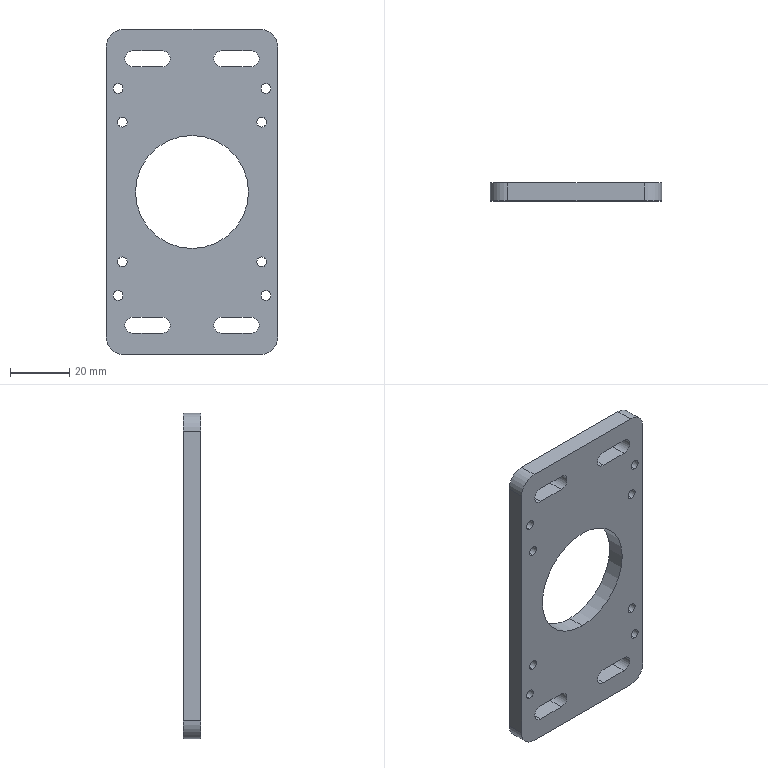Part | SolidWorks | features HoleWzd 2, Extrusion 1, ICE 1 | 1 solid | 44 faces | box 58 x 6 x 110 mm | volume 28962 mm3 | cylinder 30 | plane 14 | commonest cylinder face diameters 3.3 x16 5.4 x8 12 x4 38.2 x2
STEP:
#1=CARTESIAN_POINT('',(-25.,6.,36.65));
#2=VERTEX_POINT('',#1);
#3=CARTESIAN_POINT('',(-25.,6.,33.35));
#4=VERTEX_POINT('',#3);
#5=CARTESIAN_POINT('',(-25.,6.,35.));
#6=DIRECTION('',(0.,-1.,0.));
#7=DIRECTION('',(0.,0.,-1.));
#8=AXIS2_PLACEMENT_3D('',#5,#6,#7);
#9=CIRCLE('',#8,1.65);
#10=EDGE_CURVE('',#2,#4,#9,.T.);
#11=ORIENTED_EDGE('',*,*,#10,.F.);
#12=CARTESIAN_POINT('',(-25.,0.,36.65));
#13=VERTEX_POINT('',#12);
#14=CARTESIAN_POINT('',(-25.,0.,36.65));
#15=DIRECTION('',(0.,-1.,0.));
#16=VECTOR('',#15,1000.);
#17=LINE('',#14,#16);
#18=EDGE_CURVE('',#2,#13,#17,.T.);
#19=ORIENTED_EDGE('',*,*,#18,.T.);
#20=CARTESIAN_POINT('',(-25.,0.,33.35));
#21=VERTEX_POINT('',#20);
#22=CARTESIAN_POINT('',(-25.,0.,35.));
#23=DIRECTION('',(0.,-1.,0.));
#24=DIRECTION('',(0.,0.,-1.));
#25=AXIS2_PLACEMENT_3D('',#22,#23,#24);
#26=CIRCLE('',#25,1.65);
#27=EDGE_CURVE('',#13,#21,#26,.T.);
#28=ORIENTED_EDGE('',*,*,#27,.T.);
#29=CARTESIAN_POINT('',(-25.,0.,33.35));
#30=DIRECTION('',(0.,-1.,0.));
#31=VECTOR('',#30,1000.);
#32=LINE('',#29,#31);
#33=EDGE_CURVE('',#4,#21,#32,.T.);
#34=ORIENTED_EDGE('',*,*,#33,.F.);
#35=EDGE_LOOP('',(#11,#19,#28,#34));
#36=FACE_OUTER_BOUND('',#35,.T.);
#37=CARTESIAN_POINT('',(-25.,0.,35.));
#38=DIRECTION('',(0.,-1.,0.));
#39=DIRECTION('',(0.,0.,-1.));
#40=AXIS2_PLACEMENT_3D('',#37,#38,#39);
#41=CYLINDRICAL_SURFACE('',#40,1.65);
#42=ADVANCED_FACE('',(#36),#41,.F.);
#43=CARTESIAN_POINT('',(-25.,6.,-33.35));
#44=VERTEX_POINT('',#43);
#45=CARTESIAN_POINT('',(-25.,6.,-36.65));
#46=VERTEX_POINT('',#45);
#47=CARTESIAN_POINT('',(-25.,6.,-35.));
#48=DIRECTION('',(0.,-1.,0.));
#49=DIRECTION('',(0.,0.,-1.));
#50=AXIS2_PLACEMENT_3D('',#47,#48,#49);
#51=CIRCLE('',#50,1.65);
#52=EDGE_CURVE('',#44,#46,#51,.T.);
#53=ORIENTED_EDGE('',*,*,#52,.F.);
#54=CARTESIAN_POINT('',(-25.,0.,-33.35));
#55=VERTEX_POINT('',#54);
#56=CARTESIAN_POINT('',(-25.,0.,-33.35));
#57=DIRECTION('',(0.,-1.,0.));
#58=VECTOR('',#57,1000.);
#59=LINE('',#56,#58);
#60=EDGE_CURVE('',#44,#55,#59,.T.);
#61=ORIENTED_EDGE('',*,*,#60,.T.);
#62=CARTESIAN_POINT('',(-25.,0.,-36.65));
#63=VERTEX_POINT('',#62);
#64=CARTESIAN_POINT('',(-25.,0.,-35.));
#65=DIRECTION('',(0.,-1.,0.));
#66=DIRECTION('',(0.,0.,-1.));
#67=AXIS2_PLACEMENT_3D('',#64,#65,#66);
#68=CIRCLE('',#67,1.65);
#69=EDGE_CURVE('',#55,#63,#68,.T.);
#70=ORIENTED_EDGE('',*,*,#69,.T.);
#71=CARTESIAN_POINT('',(-25.,0.,-36.65));
#72=DIRECTION('',(0.,-1.,0.));
#73=VECTOR('',#72,1000.);
#74=LINE('',#71,#73);
#75=EDGE_CURVE('',#46,#63,#74,.T.);
#76=ORIENTED_EDGE('',*,*,#75,.F.);
#77=EDGE_LOOP('',(#53,#61,#70,#76));
#78=FACE_OUTER_BOUND('',#77,.T.);
#79=CARTESIAN_POINT('',(-25.,0.,-35.));
#80=DIRECTION('',(0.,-1.,0.));
#81=DIRECTION('',(0.,0.,-1.));
#82=AXIS2_PLACEMENT_3D('',#79,#80,#81);
#83=CYLINDRICAL_SURFACE('',#82,1.65);
#84=ADVANCED_FACE('',(#78),#83,.F.);
#85=CARTESIAN_POINT('',(25.,6.,-33.35));
#86=VERTEX_POINT('',#85);
#87=CARTESIAN_POINT('',(25.,6.,-36.65));
#88=VERTEX_POINT('',#87);
#89=CARTESIAN_POINT('',(25.,6.,-35.));
#90=DIRECTION('',(0.,-1.,0.));
#91=DIRECTION('',(0.,0.,-1.));
#92=AXIS2_PLACEMENT_3D('',#89,#90,#91);
#93=CIRCLE('',#92,1.65);
#94=EDGE_CURVE('',#86,#88,#93,.T.);
#95=ORIENTED_EDGE('',*,*,#94,.F.);
#96=CARTESIAN_POINT('',(25.,0.,-33.35));
#97=VERTEX_POINT('',#96);
#98=CARTESIAN_POINT('',(25.,0.,-33.35));
#99=DIRECTION('',(0.,-1.,0.));
#100=VECTOR('',#99,1000.);
#101=LINE('',#98,#100);
#102=EDGE_CURVE('',#86,#97,#101,.T.);
#103=ORIENTED_EDGE('',*,*,#102,.T.);
#104=CARTESIAN_POINT('',(25.,0.,-36.65));
#105=VERTEX_POINT('',#104);
#106=CARTESIAN_POINT('',(25.,0.,-35.));
#107=DIRECTION('',(0.,-1.,0.));
#108=DIRECTION('',(0.,0.,-1.));
#109=AXIS2_PLACEMENT_3D('',#106,#107,#108);
#110=CIRCLE('',#109,1.65);
#111=EDGE_CURVE('',#97,#105,#110,.T.);
#112=ORIENTED_EDGE('',*,*,#111,.T.);
#113=CARTESIAN_POINT('',(25.,0.,-36.65));
#114=DIRECTION('',(0.,-1.,0.));
#115=VECTOR('',#114,1000.);
#116=LINE('',#113,#115);
#117=EDGE_CURVE('',#88,#105,#116,.T.);
#118=ORIENTED_EDGE('',*,*,#117,.F.);
#119=EDGE_LOOP('',(#95,#103,#112,#118));
#120=FACE_OUTER_BOUND('',#119,.T.);
#121=CARTESIAN_POINT('',(25.,0.,-35.));
#122=DIRECTION('',(0.,-1.,0.));
#123=DIRECTION('',(0.,0.,-1.));
#124=AXIS2_PLACEMENT_3D('',#121,#122,#123);
#125=CYLINDRICAL_SURFACE('',#124,1.65);
#126=ADVANCED_FACE('',(#120),#125,.F.);
#127=CARTESIAN_POINT('',(25.,6.,36.65));
#128=VERTEX_POINT('',#127);
#129=CARTESIAN_POINT('',(25.,6.,33.35));
#130=VERTEX_POINT('',#129);
#131=CARTESIAN_POINT('',(25.,6.,35.));
#132=DIRECTION('',(0.,-1.,0.));
#133=DIRECTION('',(0.,0.,-1.));
#134=AXIS2_PLACEMENT_3D('',#131,#132,#133);
#135=CIRCLE('',#134,1.65);
#136=EDGE_CURVE('',#128,#130,#135,.T.);
#137=ORIENTED_EDGE('',*,*,#136,.F.);
#138=CARTESIAN_POINT('',(25.,0.,36.65));
#139=VERTEX_POINT('',#138);
#140=CARTESIAN_POINT('',(25.,0.,36.65));
#141=DIRECTION('',(0.,-1.,0.));
#142=VECTOR('',#141,1000.);
#143=LINE('',#140,#142);
#144=EDGE_CURVE('',#128,#139,#143,.T.);
#145=ORIENTED_EDGE('',*,*,#144,.T.);
#146=CARTESIAN_POINT('',(25.,0.,33.35));
#147=VERTEX_POINT('',#146);
#148=CARTESIAN_POINT('',(25.,0.,35.));
#149=DIRECTION('',(0.,-1.,0.));
#150=DIRECTION('',(0.,0.,-1.));
#151=AXIS2_PLACEMENT_3D('',#148,#149,#150);
#152=CIRCLE('',#151,1.65);
#153=EDGE_CURVE('',#139,#147,#152,.T.);
#154=ORIENTED_EDGE('',*,*,#153,.T.);
#155=CARTESIAN_POINT('',(25.,0.,33.35));
#156=DIRECTION('',(0.,-1.,0.));
#157=VECTOR('',#156,1000.);
#158=LINE('',#155,#157);
#159=EDGE_CURVE('',#130,#147,#158,.T.);
#160=ORIENTED_EDGE('',*,*,#159,.F.);
#161=EDGE_LOOP('',(#137,#145,#154,#160));
#162=FACE_OUTER_BOUND('',#161,.T.);
#163=CARTESIAN_POINT('',(25.,0.,35.));
#164=DIRECTION('',(0.,-1.,0.));
#165=DIRECTION('',(0.,0.,-1.));
#166=AXIS2_PLACEMENT_3D('',#163,#164,#165);
#167=CYLINDRICAL_SURFACE('',#166,1.65);
#168=ADVANCED_FACE('',(#162),#167,.F.);
#169=CARTESIAN_POINT('',(-23.57,0.,-21.92));
#170=VERTEX_POINT('',#169);
#171=CARTESIAN_POINT('',(-23.57,0.,-25.22));
#172=VERTEX_POINT('',#171);
#173=CARTESIAN_POINT('',(-23.57,0.,-23.57));
#174=DIRECTION('',(0.,-1.,0.));
#175=DIRECTION('',(0.,0.,-1.));
#176=AXIS2_PLACEMENT_3D('',#173,#174,#175);
#177=CIRCLE('',#176,1.65);
#178=EDGE_CURVE('',#170,#172,#177,.T.);
#179=ORIENTED_EDGE('',*,*,#178,.T.);
#180=CARTESIAN_POINT('',(-23.57,6.,-25.22));
#181=VERTEX_POINT('',#180);
#182=CARTESIAN_POINT('',(-23.57,6.,-25.22));
#183=DIRECTION('',(0.,1.,0.));
#184=VECTOR('',#183,1000.);
#185=LINE('',#182,#184);
#186=EDGE_CURVE('',#172,#181,#185,.T.);
#187=ORIENTED_EDGE('',*,*,#186,.T.);
#188=CARTESIAN_POINT('',(-23.57,6.,-21.92));
#189=VERTEX_POINT('',#188);
#190=CARTESIAN_POINT('',(-23.57,6.,-23.57));
#191=DIRECTION('',(0.,1.,0.));
#192=DIRECTION('',(0.,0.,1.));
#193=AXIS2_PLACEMENT_3D('',#190,#191,#192);
#194=CIRCLE('',#193,1.65);
#195=EDGE_CURVE('',#181,#189,#194,.T.);
#196=ORIENTED_EDGE('',*,*,#195,.T.);
#197=CARTESIAN_POINT('',(-23.57,6.,-21.92));
#198=DIRECTION('',(0.,1.,0.));
#199=VECTOR('',#198,1000.);
#200=LINE('',#197,#199);
#201=EDGE_CURVE('',#170,#189,#200,.T.);
#202=ORIENTED_EDGE('',*,*,#201,.F.);
#203=EDGE_LOOP('',(#179,#187,#196,#202));
#204=FACE_OUTER_BOUND('',#203,.T.);
#205=CARTESIAN_POINT('',(-23.57,6.,-23.57));
#206=DIRECTION('',(0.,1.,0.));
#207=DIRECTION('',(0.,0.,1.));
#208=AXIS2_PLACEMENT_3D('',#205,#206,#207);
#209=CYLINDRICAL_SURFACE('',#208,1.65);
#210=ADVANCED_FACE('',(#204),#209,.F.);
#211=CARTESIAN_POINT('',(23.57,0.,-21.92));
#212=VERTEX_POINT('',#211);
#213=CARTESIAN_POINT('',(23.57,0.,-25.22));
#214=VERTEX_POINT('',#213);
#215=CARTESIAN_POINT('',(23.57,0.,-23.57));
#216=DIRECTION('',(0.,-1.,0.));
#217=DIRECTION('',(0.,0.,-1.));
#218=AXIS2_PLACEMENT_3D('',#215,#216,#217);
#219=CIRCLE('',#218,1.65);
#220=EDGE_CURVE('',#212,#214,#219,.T.);
#221=ORIENTED_EDGE('',*,*,#220,.T.);
#222=CARTESIAN_POINT('',(23.57,6.,-25.22));
#223=VERTEX_POINT('',#222);
#224=CARTESIAN_POINT('',(23.57,6.,-25.22));
#225=DIRECTION('',(0.,1.,0.));
#226=VECTOR('',#225,1000.);
#227=LINE('',#224,#226);
#228=EDGE_CURVE('',#214,#223,#227,.T.);
#229=ORIENTED_EDGE('',*,*,#228,.T.);
#230=CARTESIAN_POINT('',(23.57,6.,-21.92));
#231=VERTEX_POINT('',#230);
#232=CARTESIAN_POINT('',(23.57,6.,-23.57));
#233=DIRECTION('',(0.,1.,0.));
#234=DIRECTION('',(0.,0.,1.));
#235=AXIS2_PLACEMENT_3D('',#232,#233,#234);
#236=CIRCLE('',#235,1.65);
#237=EDGE_CURVE('',#223,#231,#236,.T.);
#238=ORIENTED_EDGE('',*,*,#237,.T.);
#239=CARTESIAN_POINT('',(23.57,6.,-21.92));
#240=DIRECTION('',(0.,1.,0.));
#241=VECTOR('',#240,1000.);
#242=LINE('',#239,#241);
#243=EDGE_CURVE('',#212,#231,#242,.T.);
#244=ORIENTED_EDGE('',*,*,#243,.F.);
#245=EDGE_LOOP('',(#221,#229,#238,#244));
#246=FACE_OUTER_BOUND('',#245,.T.);
#247=CARTESIAN_POINT('',(23.57,6.,-23.57));
#248=DIRECTION('',(0.,1.,0.));
#249=DIRECTION('',(0.,0.,1.));
#250=AXIS2_PLACEMENT_3D('',#247,#248,#249);
#251=CYLINDRICAL_SURFACE('',#250,1.65);
#252=ADVANCED_FACE('',(#246),#251,.F.);
#253=CARTESIAN_POINT('',(23.57,0.,25.22));
#254=VERTEX_POINT('',#253);
#255=CARTESIAN_POINT('',(23.57,0.,21.92));
#256=VERTEX_POINT('',#255);
#257=CARTESIAN_POINT('',(23.57,0.,23.57));
#258=DIRECTION('',(0.,-1.,0.));
#259=DIRECTION('',(0.,0.,-1.));
#260=AXIS2_PLACEMENT_3D('',#257,#258,#259);
#261=CIRCLE('',#260,1.65);
#262=EDGE_CURVE('',#254,#256,#261,.T.);
#263=ORIENTED_EDGE('',*,*,#262,.T.);
#264=CARTESIAN_POINT('',(23.57,6.,21.92));
#265=VERTEX_POINT('',#264);
#266=CARTESIAN_POINT('',(23.57,6.,21.92));
#267=DIRECTION('',(0.,1.,0.));
#268=VECTOR('',#267,1000.);
#269=LINE('',#266,#268);
#270=EDGE_CURVE('',#256,#265,#269,.T.);
#271=ORIENTED_EDGE('',*,*,#270,.T.);
#272=CARTESIAN_POINT('',(23.57,6.,25.22));
#273=VERTEX_POINT('',#272);
#274=CARTESIAN_POINT('',(23.57,6.,23.57));
#275=DIRECTION('',(0.,1.,0.));
#276=DIRECTION('',(0.,0.,1.));
#277=AXIS2_PLACEMENT_3D('',#274,#275,#276);
#278=CIRCLE('',#277,1.65);
#279=EDGE_CURVE('',#265,#273,#278,.T.);
#280=ORIENTED_EDGE('',*,*,#279,.T.);
#281=CARTESIAN_POINT('',(23.57,6.,25.22));
#282=DIRECTION('',(0.,1.,0.));
#283=VECTOR('',#282,1000.);
#284=LINE('',#281,#283);
#285=EDGE_CURVE('',#254,#273,#284,.T.);
#286=ORIENTED_EDGE('',*,*,#285,.F.);
#287=EDGE_LOOP('',(#263,#271,#280,#286));
#288=FACE_OUTER_BOUND('',#287,.T.);
#289=CARTESIAN_POINT('',(23.57,6.,23.57));
#290=DIRECTION('',(0.,1.,0.));
#291=DIRECTION('',(0.,0.,1.));
#292=AXIS2_PLACEMENT_3D('',#289,#290,#291);
#293=CYLINDRICAL_SURFACE('',#292,1.65);
#294=ADVANCED_FACE('',(#288),#293,.F.);
#295=CARTESIAN_POINT('',(-23.57,0.,25.22));
#296=VERTEX_POINT('',#295);
#297=CARTESIAN_POINT('',(-23.57,0.,21.92));
#298=VERTEX_POINT('',#297);
#299=CARTESIAN_POINT('',(-23.57,0.,23.57));
#300=DIRECTION('',(0.,-1.,0.));
#301=DIRECTION('',(0.,0.,-1.));
#302=AXIS2_PLACEMENT_3D('',#299,#300,#301);
#303=CIRCLE('',#302,1.65);
#304=EDGE_CURVE('',#296,#298,#303,.T.);
#305=ORIENTED_EDGE('',*,*,#304,.T.);
#306=CARTESIAN_POINT('',(-23.57,6.,21.92));
#307=VERTEX_POINT('',#306);
#308=CARTESIAN_POINT('',(-23.57,6.,21.92));
#309=DIRECTION('',(0.,1.,0.));
#310=VECTOR('',#309,1000.);
#311=LINE('',#308,#310);
#312=EDGE_CURVE('',#298,#307,#311,.T.);
#313=ORIENTED_EDGE('',*,*,#312,.T.);
#314=CARTESIAN_POINT('',(-23.57,6.,25.22));
#315=VERTEX_POINT('',#314);
#316=CARTESIAN_POINT('',(-23.57,6.,23.57));
#317=DIRECTION('',(0.,1.,0.));
#318=DIRECTION('',(0.,0.,1.));
#319=AXIS2_PLACEMENT_3D('',#316,#317,#318);
#320=CIRCLE('',#319,1.65);
#321=EDGE_CURVE('',#307,#315,#320,.T.);
#322=ORIENTED_EDGE('',*,*,#321,.T.);
#323=CARTESIAN_POINT('',(-23.57,6.,25.22));
#324=DIRECTION('',(0.,1.,0.));
#325=VECTOR('',#324,1000.);
#326=LINE('',#323,#325);
#327=EDGE_CURVE('',#296,#315,#326,.T.);
#328=ORIENTED_EDGE('',*,*,#327,.F.);
#329=EDGE_LOOP('',(#305,#313,#322,#328));
#330=FACE_OUTER_BOUND('',#329,.T.);
#331=CARTESIAN_POINT('',(-23.57,6.,23.57));
#332=DIRECTION('',(0.,1.,0.));
#333=DIRECTION('',(0.,0.,1.));
#334=AXIS2_PLACEMENT_3D('',#331,#332,#333);
#335=CYLINDRICAL_SURFACE('',#334,1.65);
#336=ADVANCED_FACE('',(#330),#335,.F.);
#337=CARTESIAN_POINT('',(0.,6.,-19.1));
#338=VERTEX_POINT('',#337);
#339=CARTESIAN_POINT('',(0.,6.,19.1));
#340=VERTEX_POINT('',#339);
#341=CARTESIAN_POINT('',(0.,6.,0.));
#342=DIRECTION('',(0.,1.,0.));
#343=DIRECTION('',(0.,0.,1.));
#344=AXIS2_PLACEMENT_3D('',#341,#342,#343);
#345=CIRCLE('',#344,19.1);
#346=EDGE_CURVE('',#338,#340,#345,.T.);
#347=ORIENTED_EDGE('',*,*,#346,.T.);
#348=CARTESIAN_POINT('',(0.,0.,19.1));
#349=VERTEX_POINT('',#348);
#350=CARTESIAN_POINT('',(0.,6.,19.1));
#351=DIRECTION('',(0.,-1.,0.));
#352=VECTOR('',#351,1000.);
#353=LINE('',#350,#352);
#354=EDGE_CURVE('',#340,#349,#353,.T.);
#355=ORIENTED_EDGE('',*,*,#354,.T.);
#356=CARTESIAN_POINT('',(0.,0.,-19.1));
#357=VERTEX_POINT('',#356);
#358=CARTESIAN_POINT('',(0.,0.,0.));
#359=DIRECTION('',(0.,1.,0.));
#360=DIRECTION('',(0.,0.,1.));
#361=AXIS2_PLACEMENT_3D('',#358,#359,#360);
#362=CIRCLE('',#361,19.1);
#363=EDGE_CURVE('',#357,#349,#362,.T.);
#364=ORIENTED_EDGE('',*,*,#363,.F.);
#365=CARTESIAN_POINT('',(0.,6.,-19.1));
#366=DIRECTION('',(0.,-1.,0.));
#367=VECTOR('',#366,1000.);
#368=LINE('',#365,#367);
#369=EDGE_CURVE('',#338,#357,#368,.T.);
#370=ORIENTED_EDGE('',*,*,#369,.F.);
#371=EDGE_LOOP('',(#347,#355,#364,#370));
#372=FACE_OUTER_BOUND('',#371,.T.);
#373=CARTESIAN_POINT('',(0.,6.,0.));
#374=DIRECTION('',(0.,-1.,0.));
#375=DIRECTION('',(0.,0.,-1.));
#376=AXIS2_PLACEMENT_3D('',#373,#374,#375);
#377=CYLINDRICAL_SURFACE('',#376,19.1);
#378=ADVANCED_FACE('',(#372),#377,.F.);
#379=CARTESIAN_POINT('',(-25.,6.,35.));
#380=DIRECTION('',(0.,-1.,0.));
#381=DIRECTION('',(0.,0.,-1.));
#382=AXIS2_PLACEMENT_3D('',#379,#380,#381);
#383=CIRCLE('',#382,1.65);
#384=EDGE_CURVE('',#4,#2,#383,.T.);
#385=ORIENTED_EDGE('',*,*,#384,.T.);
#386=ORIENTED_EDGE('',*,*,#10,.T.);
#387=EDGE_LOOP('',(#385,#386));
#388=FACE_BOUND('',#387,.T.);
#389=CARTESIAN_POINT('',(-25.,6.,-35.));
#390=DIRECTION('',(0.,-1.,0.));
#391=DIRECTION('',(0.,0.,-1.));
#392=AXIS2_PLACEMENT_3D('',#389,#390,#391);
#393=CIRCLE('',#392,1.65);
#394=EDGE_CURVE('',#46,#44,#393,.T.);
#395=ORIENTED_EDGE('',*,*,#394,.T.);
#396=ORIENTED_EDGE('',*,*,#52,.T.);
#397=EDGE_LOOP('',(#395,#396));
#398=FACE_BOUND('',#397,.T.);
#399=CARTESIAN_POINT('',(25.,6.,-35.));
#400=DIRECTION('',(0.,-1.,0.));
#401=DIRECTION('',(0.,0.,-1.));
#402=AXIS2_PLACEMENT_3D('',#399,#400,#401);
#403=CIRCLE('',#402,1.65);
#404=EDGE_CURVE('',#88,#86,#403,.T.);
#405=ORIENTED_EDGE('',*,*,#404,.T.);
#406=ORIENTED_EDGE('',*,*,#94,.T.);
#407=EDGE_LOOP('',(#405,#406));
#408=FACE_BOUND('',#407,.T.);
#409=CARTESIAN_POINT('',(25.,6.,35.));
#410=DIRECTION('',(0.,-1.,0.));
#411=DIRECTION('',(0.,0.,-1.));
#412=AXIS2_PLACEMENT_3D('',#409,#410,#411);
#413=CIRCLE('',#412,1.65);
#414=EDGE_CURVE('',#130,#128,#413,.T.);
#415=ORIENTED_EDGE('',*,*,#414,.T.);
#416=ORIENTED_EDGE('',*,*,#136,.T.);
#417=EDGE_LOOP('',(#415,#416));
#418=FACE_BOUND('',#417,.T.);
#419=CARTESIAN_POINT('',(10.,6.,42.3));
#420=VERTEX_POINT('',#419);
#421=CARTESIAN_POINT('',(20.,6.,42.3));
#422=VERTEX_POINT('',#421);
#423=CARTESIAN_POINT('',(20.,6.,42.3));
#424=DIRECTION('',(1.,0.,0.));
#425=VECTOR('',#424,1000.);
#426=LINE('',#423,#425);
#427=EDGE_CURVE('',#420,#422,#426,.T.);
#428=ORIENTED_EDGE('',*,*,#427,.T.);
#429=CARTESIAN_POINT('',(20.,6.,47.7));
#430=VERTEX_POINT('',#429);
#431=CARTESIAN_POINT('',(20.,6.,45.));
#432=DIRECTION('',(0.,-1.,0.));
#433=DIRECTION('',(0.,0.,1.));
#434=AXIS2_PLACEMENT_3D('',#431,#432,#433);
#435=CIRCLE('',#434,2.7);
#436=EDGE_CURVE('',#422,#430,#435,.T.);
#437=ORIENTED_EDGE('',*,*,#436,.T.);
#438=CARTESIAN_POINT('',(10.,6.,47.7));
#439=VERTEX_POINT('',#438);
#440=CARTESIAN_POINT('',(20.,6.,47.7));
#441=DIRECTION('',(-1.,0.,0.));
#442=VECTOR('',#441,1000.);
#443=LINE('',#440,#442);
#444=EDGE_CURVE('',#430,#439,#443,.T.);
#445=ORIENTED_EDGE('',*,*,#444,.T.);
#446=CARTESIAN_POINT('',(10.,6.,45.));
#447=DIRECTION('',(0.,-1.,0.));
#448=DIRECTION('',(0.,0.,1.));
#449=AXIS2_PLACEMENT_3D('',#446,#447,#448);
#450=CIRCLE('',#449,2.7);
#451=EDGE_CURVE('',#439,#420,#450,.T.);
#452=ORIENTED_EDGE('',*,*,#451,.T.);
#453=EDGE_LOOP('',(#428,#437,#445,#452));
#454=FACE_BOUND('',#453,.T.);
#455=CARTESIAN_POINT('',(-10.,6.,-42.3));
#456=VERTEX_POINT('',#455);
#457=CARTESIAN_POINT('',(-20.,6.,-42.3));
#458=VERTEX_POINT('',#457);
#459=CARTESIAN_POINT('',(-20.,6.,-42.3));
#460=DIRECTION('',(-1.,0.,0.));
#461=VECTOR('',#460,1000.);
#462=LINE('',#459,#461);
#463=EDGE_CURVE('',#456,#458,#462,.T.);
#464=ORIENTED_EDGE('',*,*,#463,.T.);
#465=CARTESIAN_POINT('',(-20.,6.,-47.7));
#466=VERTEX_POINT('',#465);
#467=CARTESIAN_POINT('',(-20.,6.,-45.));
#468=DIRECTION('',(0.,-1.,0.));
#469=DIRECTION('',(0.,0.,1.));
#470=AXIS2_PLACEMENT_3D('',#467,#468,#469);
#471=CIRCLE('',#470,2.7);
#472=EDGE_CURVE('',#458,#466,#471,.T.);
#473=ORIENTED_EDGE('',*,*,#472,.T.);
#474=CARTESIAN_POINT('',(-10.,6.,-47.7));
#475=VERTEX_POINT('',#474);
#476=CARTESIAN_POINT('',(-20.,6.,-47.7));
#477=DIRECTION('',(1.,0.,0.));
#478=VECTOR('',#477,1000.);
#479=LINE('',#476,#478);
#480=EDGE_CURVE('',#466,#475,#479,.T.);
#481=ORIENTED_EDGE('',*,*,#480,.T.);
#482=CARTESIAN_POINT('',(-10.,6.,-45.));
#483=DIRECTION('',(0.,-1.,0.));
#484=DIRECTION('',(0.,0.,1.));
#485=AXIS2_PLACEMENT_3D('',#482,#483,#484);
#486=CIRCLE('',#485,2.7);
#487=EDGE_CURVE('',#475,#456,#486,.T.);
#488=ORIENTED_EDGE('',*,*,#487,.T.);
#489=EDGE_LOOP('',(#464,#473,#481,#488));
#490=FACE_BOUND('',#489,.T.);
#491=CARTESIAN_POINT('',(10.,6.,-47.7));
#492=VERTEX_POINT('',#491);
#493=CARTESIAN_POINT('',(20.,6.,-47.7));
#494=VERTEX_POINT('',#493);
#495=CARTESIAN_POINT('',(20.,6.,-47.7));
#496=DIRECTION('',(1.,0.,0.));
#497=VECTOR('',#496,1000.);
#498=LINE('',#495,#497);
#499=EDGE_CURVE('',#492,#494,#498,.T.);
#500=ORIENTED_EDGE('',*,*,#499,.T.);
#501=CARTESIAN_POINT('',(20.,6.,-42.3));
#502=VERTEX_POINT('',#501);
#503=CARTESIAN_POINT('',(20.,6.,-45.));
#504=DIRECTION('',(0.,-1.,0.));
#505=DIRECTION('',(0.,0.,-1.));
#506=AXIS2_PLACEMENT_3D('',#503,#504,#505);
#507=CIRCLE('',#506,2.7);
#508=EDGE_CURVE('',#494,#502,#507,.T.);
#509=ORIENTED_EDGE('',*,*,#508,.T.);
#510=CARTESIAN_POINT('',(10.,6.,-42.3));
#511=VERTEX_POINT('',#510);
#512=CARTESIAN_POINT('',(20.,6.,-42.3));
#513=DIRECTION('',(-1.,0.,0.));
#514=VECTOR('',#513,1000.);
#515=LINE('',#512,#514);
#516=EDGE_CURVE('',#502,#511,#515,.T.);
#517=ORIENTED_EDGE('',*,*,#516,.T.);
#518=CARTESIAN_POINT('',(10.,6.,-45.));
#519=DIRECTION('',(0.,-1.,0.));
#520=DIRECTION('',(0.,0.,-1.));
#521=AXIS2_PLACEMENT_3D('',#518,#519,#520);
#522=CIRCLE('',#521,2.7);
#523=EDGE_CURVE('',#511,#492,#522,.T.);
#524=ORIENTED_EDGE('',*,*,#523,.T.);
#525=EDGE_LOOP('',(#500,#509,#517,#524));
#526=FACE_BOUND('',#525,.T.);
#527=CARTESIAN_POINT('',(-10.,6.,47.7));
#528=VERTEX_POINT('',#527);
#529=CARTESIAN_POINT('',(-20.,6.,47.7));
#530=VERTEX_POINT('',#529);
#531=CARTESIAN_POINT('',(-20.,6.,47.7));
#532=DIRECTION('',(-1.,0.,0.));
#533=VECTOR('',#532,1000.);
#534=LINE('',#531,#533);
#535=EDGE_CURVE('',#528,#530,#534,.T.);
#536=ORIENTED_EDGE('',*,*,#535,.T.);
#537=CARTESIAN_POINT('',(-20.,6.,42.3));
#538=VERTEX_POINT('',#537);
#539=CARTESIAN_POINT('',(-20.,6.,45.));
#540=DIRECTION('',(0.,-1.,0.));
#541=DIRECTION('',(0.,0.,-1.));
#542=AXIS2_PLACEMENT_3D('',#539,#540,#541);
#543=CIRCLE('',#542,2.7);
#544=EDGE_CURVE('',#530,#538,#543,.T.);
#545=ORIENTED_EDGE('',*,*,#544,.T.);
#546=CARTESIAN_POINT('',(-10.,6.,42.3));
#547=VERTEX_POINT('',#546);
#548=CARTESIAN_POINT('',(-20.,6.,42.3));
#549=DIRECTION('',(1.,0.,0.));
#550=VECTOR('',#549,1000.);
#551=LINE('',#548,#550);
#552=EDGE_CURVE('',#538,#547,#551,.T.);
#553=ORIENTED_EDGE('',*,*,#552,.T.);
#554=CARTESIAN_POINT('',(-10.,6.,45.));
#555=DIRECTION('',(0.,-1.,0.));
#556=DIRECTION('',(0.,0.,-1.));
#557=AXIS2_PLACEMENT_3D('',#554,#555,#556);
#558=CIRCLE('',#557,2.7);
#559=EDGE_CURVE('',#547,#528,#558,.T.);
#560=ORIENTED_EDGE('',*,*,#559,.T.);
#561=EDGE_LOOP('',(#536,#545,#553,#560));
#562=FACE_BOUND('',#561,.T.);
#563=CARTESIAN_POINT('',(-23.57,6.,-23.57));
#564=DIRECTION('',(0.,1.,0.));
#565=DIRECTION('',(0.,0.,1.));
#566=AXIS2_PLACEMENT_3D('',#563,#564,#565);
#567=CIRCLE('',#566,1.65);
#568=EDGE_CURVE('',#189,#181,#567,.T.);
#569=ORIENTED_EDGE('',*,*,#568,.F.);
#570=ORIENTED_EDGE('',*,*,#195,.F.);
#571=EDGE_LOOP('',(#569,#570));
#572=FACE_BOUND('',#571,.T.);
#573=CARTESIAN_POINT('',(23.57,6.,-23.57));
#574=DIRECTION('',(0.,1.,0.));
#575=DIRECTION('',(0.,0.,1.));
#576=AXIS2_PLACEMENT_3D('',#573,#574,#575);
#577=CIRCLE('',#576,1.65);
#578=EDGE_CURVE('',#231,#223,#577,.T.);
#579=ORIENTED_EDGE('',*,*,#578,.F.);
#580=ORIENTED_EDGE('',*,*,#237,.F.);
#581=EDGE_LOOP('',(#579,#580));
#582=FACE_BOUND('',#581,.T.);
#583=CARTESIAN_POINT('',(23.57,6.,23.57));
#584=DIRECTION('',(0.,1.,0.));
#585=DIRECTION('',(0.,0.,1.));
#586=AXIS2_PLACEMENT_3D('',#583,#584,#585);
#587=CIRCLE('',#586,1.65);
#588=EDGE_CURVE('',#273,#265,#587,.T.);
#589=ORIENTED_EDGE('',*,*,#588,.F.);
#590=ORIENTED_EDGE('',*,*,#279,.F.);
#591=EDGE_LOOP('',(#589,#590));
#592=FACE_BOUND('',#591,.T.);
#593=CARTESIAN_POINT('',(-23.57,6.,23.57));
#594=DIRECTION('',(0.,1.,0.));
#595=DIRECTION('',(0.,0.,1.));
#596=AXIS2_PLACEMENT_3D('',#593,#594,#595);
#597=CIRCLE('',#596,1.65);
#598=EDGE_CURVE('',#315,#307,#597,.T.);
#599=ORIENTED_EDGE('',*,*,#598,.F.);
#600=ORIENTED_EDGE('',*,*,#321,.F.);
#601=EDGE_LOOP('',(#599,#600));
#602=FACE_BOUND('',#601,.T.);
#603=CARTESIAN_POINT('',(29.,6.,-49.));
#604=VERTEX_POINT('',#603);
#605=CARTESIAN_POINT('',(23.,6.,-55.));
#606=VERTEX_POINT('',#605);
#607=CARTESIAN_POINT('',(23.,6.,-49.));
#608=DIRECTION('',(0.,1.,0.));
#609=DIRECTION('',(0.,0.,-1.));
#610=AXIS2_PLACEMENT_3D('',#607,#608,#609);
#611=CIRCLE('',#610,6.);
#612=EDGE_CURVE('',#604,#606,#611,.T.);
#613=ORIENTED_EDGE('',*,*,#612,.T.);
#614=CARTESIAN_POINT('',(-23.,6.,-55.));
#615=VERTEX_POINT('',#614);
#616=CARTESIAN_POINT('',(-23.,6.,-55.));
#617=DIRECTION('',(-1.,0.,0.));
#618=VECTOR('',#617,1000.);
#619=LINE('',#616,#618);
#620=EDGE_CURVE('',#606,#615,#619,.T.);
#621=ORIENTED_EDGE('',*,*,#620,.T.);
#622=CARTESIAN_POINT('',(-29.,6.,-49.));
#623=VERTEX_POINT('',#622);
#624=CARTESIAN_POINT('',(-23.,6.,-49.));
#625=DIRECTION('',(0.,1.,0.));
#626=DIRECTION('',(0.,0.,1.));
#627=AXIS2_PLACEMENT_3D('',#624,#625,#626);
#628=CIRCLE('',#627,6.);
#629=EDGE_CURVE('',#615,#623,#628,.T.);
#630=ORIENTED_EDGE('',*,*,#629,.T.);
#631=CARTESIAN_POINT('',(-29.,6.,49.));
#632=VERTEX_POINT('',#631);
#633=CARTESIAN_POINT('',(-29.,6.,-49.));
#634=DIRECTION('',(0.,0.,1.));
#635=VECTOR('',#634,1000.);
#636=LINE('',#633,#635);
#637=EDGE_CURVE('',#623,#632,#636,.T.);
#638=ORIENTED_EDGE('',*,*,#637,.T.);
#639=CARTESIAN_POINT('',(-23.,6.,55.));
#640=VERTEX_POINT('',#639);
#641=CARTESIAN_POINT('',(-23.,6.,49.));
#642=DIRECTION('',(0.,1.,0.));
#643=DIRECTION('',(0.,0.,1.));
#644=AXIS2_PLACEMENT_3D('',#641,#642,#643);
#645=CIRCLE('',#644,6.);
#646=EDGE_CURVE('',#632,#640,#645,.T.);
#647=ORIENTED_EDGE('',*,*,#646,.T.);
#648=CARTESIAN_POINT('',(23.,6.,55.));
#649=VERTEX_POINT('',#648);
#650=CARTESIAN_POINT('',(-23.,6.,55.));
#651=DIRECTION('',(1.,0.,0.));
#652=VECTOR('',#651,1000.);
#653=LINE('',#650,#652);
#654=EDGE_CURVE('',#640,#649,#653,.T.);
#655=ORIENTED_EDGE('',*,*,#654,.T.);
#656=CARTESIAN_POINT('',(29.,6.,49.));
#657=VERTEX_POINT('',#656);
#658=CARTESIAN_POINT('',(23.,6.,49.));
#659=DIRECTION('',(0.,1.,0.));
#660=DIRECTION('',(0.,0.,1.));
#661=AXIS2_PLACEMENT_3D('',#658,#659,#660);
#662=CIRCLE('',#661,6.);
#663=EDGE_CURVE('',#649,#657,#662,.T.);
#664=ORIENTED_EDGE('',*,*,#663,.T.);
#665=CARTESIAN_POINT('',(29.,6.,-49.));
#666=DIRECTION('',(0.,0.,-1.));
#667=VECTOR('',#666,1000.);
#668=LINE('',#665,#667);
#669=EDGE_CURVE('',#657,#604,#668,.T.);
#670=ORIENTED_EDGE('',*,*,#669,.T.);
#671=EDGE_LOOP('',(#613,#621,#630,#638,#647,#655,#664,#670));
#672=FACE_OUTER_BOUND('',#671,.T.);
#673=ORIENTED_EDGE('',*,*,#346,.F.);
#674=CARTESIAN_POINT('',(0.,6.,0.));
#675=DIRECTION('',(0.,1.,0.));
#676=DIRECTION('',(0.,0.,1.));
#677=AXIS2_PLACEMENT_3D('',#674,#675,#676);
#678=CIRCLE('',#677,19.1);
#679=EDGE_CURVE('',#340,#338,#678,.T.);
#680=ORIENTED_EDGE('',*,*,#679,.F.);
#681=EDGE_LOOP('',(#673,#680));
#682=FACE_BOUND('',#681,.T.);
#683=CARTESIAN_POINT('',(23.,6.,-49.));
#684=DIRECTION('',(0.,-1.,0.));
#685=DIRECTION('',(0.,0.,-1.));
#686=AXIS2_PLACEMENT_3D('',#683,#684,#685);
#687=PLANE('',#686);
#688=ADVANCED_FACE('',(#388,#398,#408,#418,#454,#490,#526,#562,#572,#582,#592,#602,#672,#682),#687,.F.);
#689=CARTESIAN_POINT('',(-25.,0.,35.));
#690=DIRECTION('',(0.,-1.,0.));
#691=DIRECTION('',(0.,0.,-1.));
#692=AXIS2_PLACEMENT_3D('',#689,#690,#691);
#693=CIRCLE('',#692,1.65);
#694=EDGE_CURVE('',#21,#13,#693,.T.);
#695=ORIENTED_EDGE('',*,*,#694,.F.);
#696=ORIENTED_EDGE('',*,*,#27,.F.);
#697=EDGE_LOOP('',(#695,#696));
#698=FACE_BOUND('',#697,.T.);
#699=CARTESIAN_POINT('',(-25.,0.,-35.));
#700=DIRECTION('',(0.,-1.,0.));
#701=DIRECTION('',(0.,0.,-1.));
#702=AXIS2_PLACEMENT_3D('',#699,#700,#701);
#703=CIRCLE('',#702,1.65);
#704=EDGE_CURVE('',#63,#55,#703,.T.);
#705=ORIENTED_EDGE('',*,*,#704,.F.);
#706=ORIENTED_EDGE('',*,*,#69,.F.);
#707=EDGE_LOOP('',(#705,#706));
#708=FACE_BOUND('',#707,.T.);
#709=CARTESIAN_POINT('',(25.,0.,-35.));
#710=DIRECTION('',(0.,-1.,0.));
#711=DIRECTION('',(0.,0.,-1.));
#712=AXIS2_PLACEMENT_3D('',#709,#710,#711);
#713=CIRCLE('',#712,1.65);
#714=EDGE_CURVE('',#105,#97,#713,.T.);
#715=ORIENTED_EDGE('',*,*,#714,.F.);
#716=ORIENTED_EDGE('',*,*,#111,.F.);
#717=EDGE_LOOP('',(#715,#716));
#718=FACE_BOUND('',#717,.T.);
#719=CARTESIAN_POINT('',(25.,0.,35.));
#720=DIRECTION('',(0.,-1.,0.));
#721=DIRECTION('',(0.,0.,-1.));
#722=AXIS2_PLACEMENT_3D('',#719,#720,#721);
#723=CIRCLE('',#722,1.65);
#724=EDGE_CURVE('',#147,#139,#723,.T.);
#725=ORIENTED_EDGE('',*,*,#724,.F.);
#726=ORIENTED_EDGE('',*,*,#153,.F.);
#727=EDGE_LOOP('',(#725,#726));
#728=FACE_BOUND('',#727,.T.);
#729=CARTESIAN_POINT('',(20.,0.,42.3));
#730=VERTEX_POINT('',#729);
#731=CARTESIAN_POINT('',(20.,0.,47.7));
#732=VERTEX_POINT('',#731);
#733=CARTESIAN_POINT('',(20.,0.,45.));
#734=DIRECTION('',(0.,-1.,0.));
#735=DIRECTION('',(0.,0.,1.));
#736=AXIS2_PLACEMENT_3D('',#733,#734,#735);
#737=CIRCLE('',#736,2.7);
#738=EDGE_CURVE('',#730,#732,#737,.T.);
#739=ORIENTED_EDGE('',*,*,#738,.F.);
#740=CARTESIAN_POINT('',(10.,0.,42.3));
#741=VERTEX_POINT('',#740);
#742=CARTESIAN_POINT('',(20.,0.,42.3));
#743=DIRECTION('',(1.,0.,0.));
#744=VECTOR('',#743,1000.);
#745=LINE('',#742,#744);
#746=EDGE_CURVE('',#741,#730,#745,.T.);
#747=ORIENTED_EDGE('',*,*,#746,.F.);
#748=CARTESIAN_POINT('',(10.,0.,47.7));
#749=VERTEX_POINT('',#748);
#750=CARTESIAN_POINT('',(10.,0.,45.));
#751=DIRECTION('',(0.,-1.,0.));
#752=DIRECTION('',(0.,0.,1.));
#753=AXIS2_PLACEMENT_3D('',#750,#751,#752);
#754=CIRCLE('',#753,2.7);
#755=EDGE_CURVE('',#749,#741,#754,.T.);
#756=ORIENTED_EDGE('',*,*,#755,.F.);
#757=CARTESIAN_POINT('',(20.,0.,47.7));
#758=DIRECTION('',(-1.,0.,0.));
#759=VECTOR('',#758,1000.);
#760=LINE('',#757,#759);
#761=EDGE_CURVE('',#732,#749,#760,.T.);
#762=ORIENTED_EDGE('',*,*,#761,.F.);
#763=EDGE_LOOP('',(#739,#747,#756,#762));
#764=FACE_BOUND('',#763,.T.);
#765=CARTESIAN_POINT('',(-20.,0.,-42.3));
#766=VERTEX_POINT('',#765);
#767=CARTESIAN_POINT('',(-20.,0.,-47.7));
#768=VERTEX_POINT('',#767);
#769=CARTESIAN_POINT('',(-20.,0.,-45.));
#770=DIRECTION('',(0.,-1.,0.));
#771=DIRECTION('',(0.,0.,1.));
#772=AXIS2_PLACEMENT_3D('',#769,#770,#771);
#773=CIRCLE('',#772,2.7);
#774=EDGE_CURVE('',#766,#768,#773,.T.);
#775=ORIENTED_EDGE('',*,*,#774,.F.);
#776=CARTESIAN_POINT('',(-10.,0.,-42.3));
#777=VERTEX_POINT('',#776);
#778=CARTESIAN_POINT('',(-20.,0.,-42.3));
#779=DIRECTION('',(-1.,0.,0.));
#780=VECTOR('',#779,1000.);
#781=LINE('',#778,#780);
#782=EDGE_CURVE('',#777,#766,#781,.T.);
#783=ORIENTED_EDGE('',*,*,#782,.F.);
#784=CARTESIAN_POINT('',(-10.,0.,-47.7));
#785=VERTEX_POINT('',#784);
#786=CARTESIAN_POINT('',(-10.,0.,-45.));
#787=DIRECTION('',(0.,-1.,0.));
#788=DIRECTION('',(0.,0.,1.));
#789=AXIS2_PLACEMENT_3D('',#786,#787,#788);
#790=CIRCLE('',#789,2.7);
#791=EDGE_CURVE('',#785,#777,#790,.T.);
#792=ORIENTED_EDGE('',*,*,#791,.F.);
#793=CARTESIAN_POINT('',(-20.,0.,-47.7));
#794=DIRECTION('',(1.,0.,0.));
#795=VECTOR('',#794,1000.);
#796=LINE('',#793,#795);
#797=EDGE_CURVE('',#768,#785,#796,.T.);
#798=ORIENTED_EDGE('',*,*,#797,.F.);
#799=EDGE_LOOP('',(#775,#783,#792,#798));
#800=FACE_BOUND('',#799,.T.);
#801=CARTESIAN_POINT('',(20.,0.,-47.7));
#802=VERTEX_POINT('',#801);
#803=CARTESIAN_POINT('',(20.,0.,-42.3));
#804=VERTEX_POINT('',#803);
#805=CARTESIAN_POINT('',(20.,0.,-45.));
#806=DIRECTION('',(0.,-1.,0.));
#807=DIRECTION('',(0.,0.,-1.));
#808=AXIS2_PLACEMENT_3D('',#805,#806,#807);
#809=CIRCLE('',#808,2.7);
#810=EDGE_CURVE('',#802,#804,#809,.T.);
#811=ORIENTED_EDGE('',*,*,#810,.F.);
#812=CARTESIAN_POINT('',(10.,0.,-47.7));
#813=VERTEX_POINT('',#812);
#814=CARTESIAN_POINT('',(20.,0.,-47.7));
#815=DIRECTION('',(1.,0.,0.));
#816=VECTOR('',#815,1000.);
#817=LINE('',#814,#816);
#818=EDGE_CURVE('',#813,#802,#817,.T.);
#819=ORIENTED_EDGE('',*,*,#818,.F.);
#820=CARTESIAN_POINT('',(10.,0.,-42.3));
#821=VERTEX_POINT('',#820);
#822=CARTESIAN_POINT('',(10.,0.,-45.));
#823=DIRECTION('',(0.,-1.,0.));
#824=DIRECTION('',(0.,0.,-1.));
#825=AXIS2_PLACEMENT_3D('',#822,#823,#824);
#826=CIRCLE('',#825,2.7);
#827=EDGE_CURVE('',#821,#813,#826,.T.);
#828=ORIENTED_EDGE('',*,*,#827,.F.);
#829=CARTESIAN_POINT('',(20.,0.,-42.3));
#830=DIRECTION('',(-1.,0.,0.));
#831=VECTOR('',#830,1000.);
#832=LINE('',#829,#831);
#833=EDGE_CURVE('',#804,#821,#832,.T.);
#834=ORIENTED_EDGE('',*,*,#833,.F.);
#835=EDGE_LOOP('',(#811,#819,#828,#834));
#836=FACE_BOUND('',#835,.T.);
#837=CARTESIAN_POINT('',(-20.,0.,47.7));
#838=VERTEX_POINT('',#837);
#839=CARTESIAN_POINT('',(-20.,0.,42.3));
#840=VERTEX_POINT('',#839);
#841=CARTESIAN_POINT('',(-20.,0.,45.));
#842=DIRECTION('',(0.,-1.,0.));
#843=DIRECTION('',(0.,0.,-1.));
#844=AXIS2_PLACEMENT_3D('',#841,#842,#843);
#845=CIRCLE('',#844,2.7);
#846=EDGE_CURVE('',#838,#840,#845,.T.);
#847=ORIENTED_EDGE('',*,*,#846,.F.);
#848=CARTESIAN_POINT('',(-10.,0.,47.7));
#849=VERTEX_POINT('',#848);
#850=CARTESIAN_POINT('',(-20.,0.,47.7));
#851=DIRECTION('',(-1.,0.,0.));
#852=VECTOR('',#851,1000.);
#853=LINE('',#850,#852);
#854=EDGE_CURVE('',#849,#838,#853,.T.);
#855=ORIENTED_EDGE('',*,*,#854,.F.);
#856=CARTESIAN_POINT('',(-10.,0.,42.3));
#857=VERTEX_POINT('',#856);
#858=CARTESIAN_POINT('',(-10.,0.,45.));
#859=DIRECTION('',(0.,-1.,0.));
#860=DIRECTION('',(0.,0.,-1.));
#861=AXIS2_PLACEMENT_3D('',#858,#859,#860);
#862=CIRCLE('',#861,2.7);
#863=EDGE_CURVE('',#857,#849,#862,.T.);
#864=ORIENTED_EDGE('',*,*,#863,.F.);
#865=CARTESIAN_POINT('',(-20.,0.,42.3));
#866=DIRECTION('',(1.,0.,0.));
#867=VECTOR('',#866,1000.);
#868=LINE('',#865,#867);
#869=EDGE_CURVE('',#840,#857,#868,.T.);
#870=ORIENTED_EDGE('',*,*,#869,.F.);
#871=EDGE_LOOP('',(#847,#855,#864,#870));
#872=FACE_BOUND('',#871,.T.);
#873=ORIENTED_EDGE('',*,*,#178,.F.);
#874=CARTESIAN_POINT('',(-23.57,0.,-23.57));
#875=DIRECTION('',(0.,-1.,0.));
#876=DIRECTION('',(0.,0.,-1.));
#877=AXIS2_PLACEMENT_3D('',#874,#875,#876);
#878=CIRCLE('',#877,1.65);
#879=EDGE_CURVE('',#172,#170,#878,.T.);
#880=ORIENTED_EDGE('',*,*,#879,.F.);
#881=EDGE_LOOP('',(#873,#880));
#882=FACE_BOUND('',#881,.T.);
#883=ORIENTED_EDGE('',*,*,#220,.F.);
#884=CARTESIAN_POINT('',(23.57,0.,-23.57));
#885=DIRECTION('',(0.,-1.,0.));
#886=DIRECTION('',(0.,0.,-1.));
#887=AXIS2_PLACEMENT_3D('',#884,#885,#886);
#888=CIRCLE('',#887,1.65);
#889=EDGE_CURVE('',#214,#212,#888,.T.);
#890=ORIENTED_EDGE('',*,*,#889,.F.);
#891=EDGE_LOOP('',(#883,#890));
#892=FACE_BOUND('',#891,.T.);
#893=ORIENTED_EDGE('',*,*,#262,.F.);
#894=CARTESIAN_POINT('',(23.57,0.,23.57));
#895=DIRECTION('',(0.,-1.,0.));
#896=DIRECTION('',(0.,0.,-1.));
#897=AXIS2_PLACEMENT_3D('',#894,#895,#896);
#898=CIRCLE('',#897,1.65);
#899=EDGE_CURVE('',#256,#254,#898,.T.);
#900=ORIENTED_EDGE('',*,*,#899,.F.);
#901=EDGE_LOOP('',(#893,#900));
#902=FACE_BOUND('',#901,.T.);
#903=ORIENTED_EDGE('',*,*,#304,.F.);
#904=CARTESIAN_POINT('',(-23.57,0.,23.57));
#905=DIRECTION('',(0.,-1.,0.));
#906=DIRECTION('',(0.,0.,-1.));
#907=AXIS2_PLACEMENT_3D('',#904,#905,#906);
#908=CIRCLE('',#907,1.65);
#909=EDGE_CURVE('',#298,#296,#908,.T.);
#910=ORIENTED_EDGE('',*,*,#909,.F.);
#911=EDGE_LOOP('',(#903,#910));
#912=FACE_BOUND('',#911,.T.);
#913=CARTESIAN_POINT('',(29.,0.,-49.));
#914=VERTEX_POINT('',#913);
#915=CARTESIAN_POINT('',(23.,0.,-55.));
#916=VERTEX_POINT('',#915);
#917=CARTESIAN_POINT('',(23.,0.,-49.));
#918=DIRECTION('',(0.,1.,0.));
#919=DIRECTION('',(0.,0.,-1.));
#920=AXIS2_PLACEMENT_3D('',#917,#918,#919);
#921=CIRCLE('',#920,6.);
#922=EDGE_CURVE('',#914,#916,#921,.T.);
#923=ORIENTED_EDGE('',*,*,#922,.F.);
#924=CARTESIAN_POINT('',(29.,0.,49.));
#925=VERTEX_POINT('',#924);
#926=CARTESIAN_POINT('',(29.,0.,-49.));
#927=DIRECTION('',(0.,0.,-1.));
#928=VECTOR('',#927,1000.);
#929=LINE('',#926,#928);
#930=EDGE_CURVE('',#925,#914,#929,.T.);
#931=ORIENTED_EDGE('',*,*,#930,.F.);
#932=CARTESIAN_POINT('',(23.,0.,55.));
#933=VERTEX_POINT('',#932);
#934=CARTESIAN_POINT('',(23.,0.,49.));
#935=DIRECTION('',(0.,1.,0.));
#936=DIRECTION('',(0.,0.,1.));
#937=AXIS2_PLACEMENT_3D('',#934,#935,#936);
#938=CIRCLE('',#937,6.);
#939=EDGE_CURVE('',#933,#925,#938,.T.);
#940=ORIENTED_EDGE('',*,*,#939,.F.);
#941=CARTESIAN_POINT('',(-23.,0.,55.));
#942=VERTEX_POINT('',#941);
#943=CARTESIAN_POINT('',(-23.,0.,55.));
#944=DIRECTION('',(1.,0.,0.));
#945=VECTOR('',#944,1000.);
#946=LINE('',#943,#945);
#947=EDGE_CURVE('',#942,#933,#946,.T.);
#948=ORIENTED_EDGE('',*,*,#947,.F.);
#949=CARTESIAN_POINT('',(-29.,0.,49.));
#950=VERTEX_POINT('',#949);
#951=CARTESIAN_POINT('',(-23.,0.,49.));
#952=DIRECTION('',(0.,1.,0.));
#953=DIRECTION('',(0.,0.,1.));
#954=AXIS2_PLACEMENT_3D('',#951,#952,#953);
#955=CIRCLE('',#954,6.);
#956=EDGE_CURVE('',#950,#942,#955,.T.);
#957=ORIENTED_EDGE('',*,*,#956,.F.);
#958=CARTESIAN_POINT('',(-29.,0.,-49.));
#959=VERTEX_POINT('',#958);
#960=CARTESIAN_POINT('',(-29.,0.,-49.));
#961=DIRECTION('',(0.,0.,1.));
#962=VECTOR('',#961,1000.);
#963=LINE('',#960,#962);
#964=EDGE_CURVE('',#959,#950,#963,.T.);
#965=ORIENTED_EDGE('',*,*,#964,.F.);
#966=CARTESIAN_POINT('',(-23.,0.,-55.));
#967=VERTEX_POINT('',#966);
#968=CARTESIAN_POINT('',(-23.,0.,-49.));
#969=DIRECTION('',(0.,1.,0.));
#970=DIRECTION('',(0.,0.,1.));
#971=AXIS2_PLACEMENT_3D('',#968,#969,#970);
#972=CIRCLE('',#971,6.);
#973=EDGE_CURVE('',#967,#959,#972,.T.);
#974=ORIENTED_EDGE('',*,*,#973,.F.);
#975=CARTESIAN_POINT('',(-23.,0.,-55.));
#976=DIRECTION('',(-1.,0.,0.));
#977=VECTOR('',#976,1000.);
#978=LINE('',#975,#977);
#979=EDGE_CURVE('',#916,#967,#978,.T.);
#980=ORIENTED_EDGE('',*,*,#979,.F.);
#981=EDGE_LOOP('',(#923,#931,#940,#948,#957,#965,#974,#980));
#982=FACE_OUTER_BOUND('',#981,.T.);
#983=ORIENTED_EDGE('',*,*,#363,.T.);
#984=CARTESIAN_POINT('',(0.,0.,0.));
#985=DIRECTION('',(0.,1.,0.));
#986=DIRECTION('',(0.,0.,1.));
#987=AXIS2_PLACEMENT_3D('',#984,#985,#986);
#988=CIRCLE('',#987,19.1);
#989=EDGE_CURVE('',#349,#357,#988,.T.);
#990=ORIENTED_EDGE('',*,*,#989,.T.);
#991=EDGE_LOOP('',(#983,#990));
#992=FACE_BOUND('',#991,.T.);
#993=CARTESIAN_POINT('',(23.,0.,-49.));
#994=DIRECTION('',(0.,-1.,0.));
#995=DIRECTION('',(0.,0.,-1.));
#996=AXIS2_PLACEMENT_3D('',#993,#994,#995);
#997=PLANE('',#996);
#998=ADVANCED_FACE('',(#698,#708,#718,#728,#764,#800,#836,#872,#882,#892,#902,#912,#982,#992),#997,.T.);
#999=ORIENTED_EDGE('',*,*,#922,.T.);
#1000=CARTESIAN_POINT('',(23.,6.,-55.));
#1001=DIRECTION('',(0.,-1.,0.));
#1002=VECTOR('',#1001,1000.);
#1003=LINE('',#1000,#1002);
#1004=EDGE_CURVE('',#606,#916,#1003,.T.);
#1005=ORIENTED_EDGE('',*,*,#1004,.F.);
#1006=ORIENTED_EDGE('',*,*,#612,.F.);
#1007=CARTESIAN_POINT('',(29.,6.,-49.));
#1008=DIRECTION('',(0.,-1.,0.));
#1009=VECTOR('',#1008,1000.);
#1010=LINE('',#1007,#1009);
#1011=EDGE_CURVE('',#604,#914,#1010,.T.);
#1012=ORIENTED_EDGE('',*,*,#1011,.T.);
#1013=EDGE_LOOP('',(#999,#1005,#1006,#1012));
#1014=FACE_OUTER_BOUND('',#1013,.T.);
#1015=CARTESIAN_POINT('',(23.,6.,-49.));
#1016=DIRECTION('',(0.,-1.,0.));
#1017=DIRECTION('',(0.,0.,-1.));
#1018=AXIS2_PLACEMENT_3D('',#1015,#1016,#1017);
#1019=CYLINDRICAL_SURFACE('',#1018,6.);
#1020=ADVANCED_FACE('',(#1014),#1019,.T.);
#1021=ORIENTED_EDGE('',*,*,#979,.T.);
#1022=CARTESIAN_POINT('',(-23.,6.,-55.));
#1023=DIRECTION('',(0.,-1.,0.));
#1024=VECTOR('',#1023,1000.);
#1025=LINE('',#1022,#1024);
#1026=EDGE_CURVE('',#615,#967,#1025,.T.);
#1027=ORIENTED_EDGE('',*,*,#1026,.F.);
#1028=ORIENTED_EDGE('',*,*,#620,.F.);
#1029=ORIENTED_EDGE('',*,*,#1004,.T.);
#1030=EDGE_LOOP('',(#1021,#1027,#1028,#1029));
#1031=FACE_OUTER_BOUND('',#1030,.T.);
#1032=CARTESIAN_POINT('',(-23.,6.,-55.));
#1033=DIRECTION('',(0.,0.,1.));
#1034=DIRECTION('',(1.,0.,0.));
#1035=AXIS2_PLACEMENT_3D('',#1032,#1033,#1034);
#1036=PLANE('',#1035);
#1037=ADVANCED_FACE('',(#1031),#1036,.F.);
#1038=ORIENTED_EDGE('',*,*,#973,.T.);
#1039=CARTESIAN_POINT('',(-29.,6.,-49.));
#1040=DIRECTION('',(0.,-1.,0.));
#1041=VECTOR('',#1040,1000.);
#1042=LINE('',#1039,#1041);
#1043=EDGE_CURVE('',#623,#959,#1042,.T.);
#1044=ORIENTED_EDGE('',*,*,#1043,.F.);
#1045=ORIENTED_EDGE('',*,*,#629,.F.);
#1046=ORIENTED_EDGE('',*,*,#1026,.T.);
#1047=EDGE_LOOP('',(#1038,#1044,#1045,#1046));
#1048=FACE_OUTER_BOUND('',#1047,.T.);
#1049=CARTESIAN_POINT('',(-23.,6.,-49.));
#1050=DIRECTION('',(0.,-1.,0.));
#1051=DIRECTION('',(0.,0.,-1.));
#1052=AXIS2_PLACEMENT_3D('',#1049,#1050,#1051);
#1053=CYLINDRICAL_SURFACE('',#1052,6.);
#1054=ADVANCED_FACE('',(#1048),#1053,.T.);
#1055=ORIENTED_EDGE('',*,*,#964,.T.);
#1056=CARTESIAN_POINT('',(-29.,6.,49.));
#1057=DIRECTION('',(0.,-1.,0.));
#1058=VECTOR('',#1057,1000.);
#1059=LINE('',#1056,#1058);
#1060=EDGE_CURVE('',#632,#950,#1059,.T.);
#1061=ORIENTED_EDGE('',*,*,#1060,.F.);
#1062=ORIENTED_EDGE('',*,*,#637,.F.);
#1063=ORIENTED_EDGE('',*,*,#1043,.T.);
#1064=EDGE_LOOP('',(#1055,#1061,#1062,#1063));
#1065=FACE_OUTER_BOUND('',#1064,.T.);
#1066=CARTESIAN_POINT('',(-29.,6.,-49.));
#1067=DIRECTION('',(1.,0.,0.));
#1068=DIRECTION('',(0.,0.,-1.));
#1069=AXIS2_PLACEMENT_3D('',#1066,#1067,#1068);
#1070=PLANE('',#1069);
#1071=ADVANCED_FACE('',(#1065),#1070,.F.);
#1072=ORIENTED_EDGE('',*,*,#956,.T.);
#1073=CARTESIAN_POINT('',(-23.,6.,55.));
#1074=DIRECTION('',(0.,-1.,0.));
#1075=VECTOR('',#1074,1000.);
#1076=LINE('',#1073,#1075);
#1077=EDGE_CURVE('',#640,#942,#1076,.T.);
#1078=ORIENTED_EDGE('',*,*,#1077,.F.);
#1079=ORIENTED_EDGE('',*,*,#646,.F.);
#1080=ORIENTED_EDGE('',*,*,#1060,.T.);
#1081=EDGE_LOOP('',(#1072,#1078,#1079,#1080));
#1082=FACE_OUTER_BOUND('',#1081,.T.);
#1083=CARTESIAN_POINT('',(-23.,6.,49.));
#1084=DIRECTION('',(0.,-1.,0.));
#1085=DIRECTION('',(0.,0.,-1.));
#1086=AXIS2_PLACEMENT_3D('',#1083,#1084,#1085);
#1087=CYLINDRICAL_SURFACE('',#1086,6.);
#1088=ADVANCED_FACE('',(#1082),#1087,.T.);
#1089=ORIENTED_EDGE('',*,*,#947,.T.);
#1090=CARTESIAN_POINT('',(23.,6.,55.));
#1091=DIRECTION('',(0.,-1.,0.));
#1092=VECTOR('',#1091,1000.);
#1093=LINE('',#1090,#1092);
#1094=EDGE_CURVE('',#649,#933,#1093,.T.);
#1095=ORIENTED_EDGE('',*,*,#1094,.F.);
#1096=ORIENTED_EDGE('',*,*,#654,.F.);
#1097=ORIENTED_EDGE('',*,*,#1077,.T.);
#1098=EDGE_LOOP('',(#1089,#1095,#1096,#1097));
#1099=FACE_OUTER_BOUND('',#1098,.T.);
#1100=CARTESIAN_POINT('',(-23.,6.,55.));
#1101=DIRECTION('',(0.,0.,-1.));
#1102=DIRECTION('',(-1.,0.,0.));
#1103=AXIS2_PLACEMENT_3D('',#1100,#1101,#1102);
#1104=PLANE('',#1103);
#1105=ADVANCED_FACE('',(#1099),#1104,.F.);
#1106=ORIENTED_EDGE('',*,*,#939,.T.);
#1107=CARTESIAN_POINT('',(29.,6.,49.));
#1108=DIRECTION('',(0.,-1.,0.));
#1109=VECTOR('',#1108,1000.);
#1110=LINE('',#1107,#1109);
#1111=EDGE_CURVE('',#657,#925,#1110,.T.);
#1112=ORIENTED_EDGE('',*,*,#1111,.F.);
#1113=ORIENTED_EDGE('',*,*,#663,.F.);
#1114=ORIENTED_EDGE('',*,*,#1094,.T.);
#1115=EDGE_LOOP('',(#1106,#1112,#1113,#1114));
#1116=FACE_OUTER_BOUND('',#1115,.T.);
#1117=CARTESIAN_POINT('',(23.,6.,49.));
#1118=DIRECTION('',(0.,-1.,0.));
#1119=DIRECTION('',(0.,0.,-1.));
#1120=AXIS2_PLACEMENT_3D('',#1117,#1118,#1119);
#1121=CYLINDRICAL_SURFACE('',#1120,6.);
#1122=ADVANCED_FACE('',(#1116),#1121,.T.);
#1123=ORIENTED_EDGE('',*,*,#930,.T.);
#1124=ORIENTED_EDGE('',*,*,#1011,.F.);
#1125=ORIENTED_EDGE('',*,*,#669,.F.);
#1126=ORIENTED_EDGE('',*,*,#1111,.T.);
#1127=EDGE_LOOP('',(#1123,#1124,#1125,#1126));
#1128=FACE_OUTER_BOUND('',#1127,.T.);
#1129=CARTESIAN_POINT('',(29.,6.,-49.));
#1130=DIRECTION('',(-1.,0.,0.));
#1131=DIRECTION('',(0.,0.,1.));
#1132=AXIS2_PLACEMENT_3D('',#1129,#1130,#1131);
#1133=PLANE('',#1132);
#1134=ADVANCED_FACE('',(#1128),#1133,.F.);
#1135=ORIENTED_EDGE('',*,*,#354,.F.);
#1136=ORIENTED_EDGE('',*,*,#679,.T.);
#1137=ORIENTED_EDGE('',*,*,#369,.T.);
#1138=ORIENTED_EDGE('',*,*,#989,.F.);
#1139=EDGE_LOOP('',(#1135,#1136,#1137,#1138));
#1140=FACE_OUTER_BOUND('',#1139,.T.);
#1141=CARTESIAN_POINT('',(0.,6.,0.));
#1142=DIRECTION('',(0.,-1.,0.));
#1143=DIRECTION('',(0.,0.,-1.));
#1144=AXIS2_PLACEMENT_3D('',#1141,#1142,#1143);
#1145=CYLINDRICAL_SURFACE('',#1144,19.1);
#1146=ADVANCED_FACE('',(#1140),#1145,.F.);
#1147=ORIENTED_EDGE('',*,*,#312,.F.);
#1148=ORIENTED_EDGE('',*,*,#909,.T.);
#1149=ORIENTED_EDGE('',*,*,#327,.T.);
#1150=ORIENTED_EDGE('',*,*,#598,.T.);
#1151=EDGE_LOOP('',(#1147,#1148,#1149,#1150));
#1152=FACE_OUTER_BOUND('',#1151,.T.);
#1153=CARTESIAN_POINT('',(-23.57,6.,23.57));
#1154=DIRECTION('',(0.,1.,0.));
#1155=DIRECTION('',(0.,0.,1.));
#1156=AXIS2_PLACEMENT_3D('',#1153,#1154,#1155);
#1157=CYLINDRICAL_SURFACE('',#1156,1.65);
#1158=ADVANCED_FACE('',(#1152),#1157,.F.);
#1159=ORIENTED_EDGE('',*,*,#270,.F.);
#1160=ORIENTED_EDGE('',*,*,#899,.T.);
#1161=ORIENTED_EDGE('',*,*,#285,.T.);
#1162=ORIENTED_EDGE('',*,*,#588,.T.);
#1163=EDGE_LOOP('',(#1159,#1160,#1161,#1162));
#1164=FACE_OUTER_BOUND('',#1163,.T.);
#1165=CARTESIAN_POINT('',(23.57,6.,23.57));
#1166=DIRECTION('',(0.,1.,0.));
#1167=DIRECTION('',(0.,0.,1.));
#1168=AXIS2_PLACEMENT_3D('',#1165,#1166,#1167);
#1169=CYLINDRICAL_SURFACE('',#1168,1.65);
#1170=ADVANCED_FACE('',(#1164),#1169,.F.);
#1171=ORIENTED_EDGE('',*,*,#228,.F.);
#1172=ORIENTED_EDGE('',*,*,#889,.T.);
#1173=ORIENTED_EDGE('',*,*,#243,.T.);
#1174=ORIENTED_EDGE('',*,*,#578,.T.);
#1175=EDGE_LOOP('',(#1171,#1172,#1173,#1174));
#1176=FACE_OUTER_BOUND('',#1175,.T.);
#1177=CARTESIAN_POINT('',(23.57,6.,-23.57));
#1178=DIRECTION('',(0.,1.,0.));
#1179=DIRECTION('',(0.,0.,1.));
#1180=AXIS2_PLACEMENT_3D('',#1177,#1178,#1179);
#1181=CYLINDRICAL_SURFACE('',#1180,1.65);
#1182=ADVANCED_FACE('',(#1176),#1181,.F.);
#1183=ORIENTED_EDGE('',*,*,#186,.F.);
#1184=ORIENTED_EDGE('',*,*,#879,.T.);
#1185=ORIENTED_EDGE('',*,*,#201,.T.);
#1186=ORIENTED_EDGE('',*,*,#568,.T.);
#1187=EDGE_LOOP('',(#1183,#1184,#1185,#1186));
#1188=FACE_OUTER_BOUND('',#1187,.T.);
#1189=CARTESIAN_POINT('',(-23.57,6.,-23.57));
#1190=DIRECTION('',(0.,1.,0.));
#1191=DIRECTION('',(0.,0.,1.));
#1192=AXIS2_PLACEMENT_3D('',#1189,#1190,#1191);
#1193=CYLINDRICAL_SURFACE('',#1192,1.65);
#1194=ADVANCED_FACE('',(#1188),#1193,.F.);
#1195=ORIENTED_EDGE('',*,*,#846,.T.);
#1196=CARTESIAN_POINT('',(-20.,6.,42.3));
#1197=DIRECTION('',(0.,-1.,0.));
#1198=VECTOR('',#1197,1000.);
#1199=LINE('',#1196,#1198);
#1200=EDGE_CURVE('',#538,#840,#1199,.T.);
#1201=ORIENTED_EDGE('',*,*,#1200,.F.);
#1202=ORIENTED_EDGE('',*,*,#544,.F.);
#1203=CARTESIAN_POINT('',(-20.,6.,47.7));
#1204=DIRECTION('',(0.,-1.,0.));
#1205=VECTOR('',#1204,1000.);
#1206=LINE('',#1203,#1205);
#1207=EDGE_CURVE('',#530,#838,#1206,.T.);
#1208=ORIENTED_EDGE('',*,*,#1207,.T.);
#1209=EDGE_LOOP('',(#1195,#1201,#1202,#1208));
#1210=FACE_OUTER_BOUND('',#1209,.T.);
#1211=CARTESIAN_POINT('',(-20.,6.,45.));
#1212=DIRECTION('',(0.,-1.,0.));
#1213=DIRECTION('',(0.,0.,-1.));
#1214=AXIS2_PLACEMENT_3D('',#1211,#1212,#1213);
#1215=CYLINDRICAL_SURFACE('',#1214,2.7);
#1216=ADVANCED_FACE('',(#1210),#1215,.F.);
#1217=ORIENTED_EDGE('',*,*,#854,.T.);
#1218=ORIENTED_EDGE('',*,*,#1207,.F.);
#1219=ORIENTED_EDGE('',*,*,#535,.F.);
#1220=CARTESIAN_POINT('',(-10.,6.,47.7));
#1221=DIRECTION('',(0.,-1.,0.));
#1222=VECTOR('',#1221,1000.);
#1223=LINE('',#1220,#1222);
#1224=EDGE_CURVE('',#528,#849,#1223,.T.);
#1225=ORIENTED_EDGE('',*,*,#1224,.T.);
#1226=EDGE_LOOP('',(#1217,#1218,#1219,#1225));
#1227=FACE_OUTER_BOUND('',#1226,.T.);
#1228=CARTESIAN_POINT('',(-20.,6.,47.7));
#1229=DIRECTION('',(0.,0.,1.));
#1230=DIRECTION('',(1.,0.,0.));
#1231=AXIS2_PLACEMENT_3D('',#1228,#1229,#1230);
#1232=PLANE('',#1231);
#1233=ADVANCED_FACE('',(#1227),#1232,.F.);
#1234=ORIENTED_EDGE('',*,*,#863,.T.);
#1235=ORIENTED_EDGE('',*,*,#1224,.F.);
#1236=ORIENTED_EDGE('',*,*,#559,.F.);
#1237=CARTESIAN_POINT('',(-10.,6.,42.3));
#1238=DIRECTION('',(0.,-1.,0.));
#1239=VECTOR('',#1238,1000.);
#1240=LINE('',#1237,#1239);
#1241=EDGE_CURVE('',#547,#857,#1240,.T.);
#1242=ORIENTED_EDGE('',*,*,#1241,.T.);
#1243=EDGE_LOOP('',(#1234,#1235,#1236,#1242));
#1244=FACE_OUTER_BOUND('',#1243,.T.);
#1245=CARTESIAN_POINT('',(-10.,6.,45.));
#1246=DIRECTION('',(0.,-1.,0.));
#1247=DIRECTION('',(0.,0.,-1.));
#1248=AXIS2_PLACEMENT_3D('',#1245,#1246,#1247);
#1249=CYLINDRICAL_SURFACE('',#1248,2.7);
#1250=ADVANCED_FACE('',(#1244),#1249,.F.);
#1251=ORIENTED_EDGE('',*,*,#869,.T.);
#1252=ORIENTED_EDGE('',*,*,#1241,.F.);
#1253=ORIENTED_EDGE('',*,*,#552,.F.);
#1254=ORIENTED_EDGE('',*,*,#1200,.T.);
#1255=EDGE_LOOP('',(#1251,#1252,#1253,#1254));
#1256=FACE_OUTER_BOUND('',#1255,.T.);
#1257=CARTESIAN_POINT('',(-20.,6.,42.3));
#1258=DIRECTION('',(0.,0.,-1.));
#1259=DIRECTION('',(-1.,0.,0.));
#1260=AXIS2_PLACEMENT_3D('',#1257,#1258,#1259);
#1261=PLANE('',#1260);
#1262=ADVANCED_FACE('',(#1256),#1261,.F.);
#1263=ORIENTED_EDGE('',*,*,#810,.T.);
#1264=CARTESIAN_POINT('',(20.,6.,-42.3));
#1265=DIRECTION('',(0.,-1.,0.));
#1266=VECTOR('',#1265,1000.);
#1267=LINE('',#1264,#1266);
#1268=EDGE_CURVE('',#502,#804,#1267,.T.);
#1269=ORIENTED_EDGE('',*,*,#1268,.F.);
#1270=ORIENTED_EDGE('',*,*,#508,.F.);
#1271=CARTESIAN_POINT('',(20.,6.,-47.7));
#1272=DIRECTION('',(0.,-1.,0.));
#1273=VECTOR('',#1272,1000.);
#1274=LINE('',#1271,#1273);
#1275=EDGE_CURVE('',#494,#802,#1274,.T.);
#1276=ORIENTED_EDGE('',*,*,#1275,.T.);
#1277=EDGE_LOOP('',(#1263,#1269,#1270,#1276));
#1278=FACE_OUTER_BOUND('',#1277,.T.);
#1279=CARTESIAN_POINT('',(20.,6.,-45.));
#1280=DIRECTION('',(0.,-1.,0.));
#1281=DIRECTION('',(0.,0.,-1.));
#1282=AXIS2_PLACEMENT_3D('',#1279,#1280,#1281);
#1283=CYLINDRICAL_SURFACE('',#1282,2.7);
#1284=ADVANCED_FACE('',(#1278),#1283,.F.);
#1285=ORIENTED_EDGE('',*,*,#818,.T.);
#1286=ORIENTED_EDGE('',*,*,#1275,.F.);
#1287=ORIENTED_EDGE('',*,*,#499,.F.);
#1288=CARTESIAN_POINT('',(10.,6.,-47.7));
#1289=DIRECTION('',(0.,-1.,0.));
#1290=VECTOR('',#1289,1000.);
#1291=LINE('',#1288,#1290);
#1292=EDGE_CURVE('',#492,#813,#1291,.T.);
#1293=ORIENTED_EDGE('',*,*,#1292,.T.);
#1294=EDGE_LOOP('',(#1285,#1286,#1287,#1293));
#1295=FACE_OUTER_BOUND('',#1294,.T.);
#1296=CARTESIAN_POINT('',(20.,6.,-47.7));
#1297=DIRECTION('',(0.,0.,-1.));
#1298=DIRECTION('',(-1.,0.,0.));
#1299=AXIS2_PLACEMENT_3D('',#1296,#1297,#1298);
#1300=PLANE('',#1299);
#1301=ADVANCED_FACE('',(#1295),#1300,.F.);
#1302=ORIENTED_EDGE('',*,*,#827,.T.);
#1303=ORIENTED_EDGE('',*,*,#1292,.F.);
#1304=ORIENTED_EDGE('',*,*,#523,.F.);
#1305=CARTESIAN_POINT('',(10.,6.,-42.3));
#1306=DIRECTION('',(0.,-1.,0.));
#1307=VECTOR('',#1306,1000.);
#1308=LINE('',#1305,#1307);
#1309=EDGE_CURVE('',#511,#821,#1308,.T.);
#1310=ORIENTED_EDGE('',*,*,#1309,.T.);
#1311=EDGE_LOOP('',(#1302,#1303,#1304,#1310));
#1312=FACE_OUTER_BOUND('',#1311,.T.);
#1313=CARTESIAN_POINT('',(10.,6.,-45.));
#1314=DIRECTION('',(0.,-1.,0.));
#1315=DIRECTION('',(0.,0.,-1.));
#1316=AXIS2_PLACEMENT_3D('',#1313,#1314,#1315);
#1317=CYLINDRICAL_SURFACE('',#1316,2.7);
#1318=ADVANCED_FACE('',(#1312),#1317,.F.);
#1319=ORIENTED_EDGE('',*,*,#833,.T.);
#1320=ORIENTED_EDGE('',*,*,#1309,.F.);
#1321=ORIENTED_EDGE('',*,*,#516,.F.);
#1322=ORIENTED_EDGE('',*,*,#1268,.T.);
#1323=EDGE_LOOP('',(#1319,#1320,#1321,#1322));
#1324=FACE_OUTER_BOUND('',#1323,.T.);
#1325=CARTESIAN_POINT('',(20.,6.,-42.3));
#1326=DIRECTION('',(0.,0.,1.));
#1327=DIRECTION('',(1.,0.,0.));
#1328=AXIS2_PLACEMENT_3D('',#1325,#1326,#1327);
#1329=PLANE('',#1328);
#1330=ADVANCED_FACE('',(#1324),#1329,.F.);
#1331=ORIENTED_EDGE('',*,*,#774,.T.);
#1332=CARTESIAN_POINT('',(-20.,6.,-47.7));
#1333=DIRECTION('',(0.,-1.,0.));
#1334=VECTOR('',#1333,1000.);
#1335=LINE('',#1332,#1334);
#1336=EDGE_CURVE('',#466,#768,#1335,.T.);
#1337=ORIENTED_EDGE('',*,*,#1336,.F.);
#1338=ORIENTED_EDGE('',*,*,#472,.F.);
#1339=CARTESIAN_POINT('',(-20.,6.,-42.3));
#1340=DIRECTION('',(0.,-1.,0.));
#1341=VECTOR('',#1340,1000.);
#1342=LINE('',#1339,#1341);
#1343=EDGE_CURVE('',#458,#766,#1342,.T.);
#1344=ORIENTED_EDGE('',*,*,#1343,.T.);
#1345=EDGE_LOOP('',(#1331,#1337,#1338,#1344));
#1346=FACE_OUTER_BOUND('',#1345,.T.);
#1347=CARTESIAN_POINT('',(-20.,6.,-45.));
#1348=DIRECTION('',(0.,-1.,0.));
#1349=DIRECTION('',(0.,0.,-1.));
#1350=AXIS2_PLACEMENT_3D('',#1347,#1348,#1349);
#1351=CYLINDRICAL_SURFACE('',#1350,2.7);
#1352=ADVANCED_FACE('',(#1346),#1351,.F.);
#1353=ORIENTED_EDGE('',*,*,#782,.T.);
#1354=ORIENTED_EDGE('',*,*,#1343,.F.);
#1355=ORIENTED_EDGE('',*,*,#463,.F.);
#1356=CARTESIAN_POINT('',(-10.,6.,-42.3));
#1357=DIRECTION('',(0.,-1.,0.));
#1358=VECTOR('',#1357,1000.);
#1359=LINE('',#1356,#1358);
#1360=EDGE_CURVE('',#456,#777,#1359,.T.);
#1361=ORIENTED_EDGE('',*,*,#1360,.T.);
#1362=EDGE_LOOP('',(#1353,#1354,#1355,#1361));
#1363=FACE_OUTER_BOUND('',#1362,.T.);
#1364=CARTESIAN_POINT('',(-20.,6.,-42.3));
#1365=DIRECTION('',(0.,0.,1.));
#1366=DIRECTION('',(1.,0.,0.));
#1367=AXIS2_PLACEMENT_3D('',#1364,#1365,#1366);
#1368=PLANE('',#1367);
#1369=ADVANCED_FACE('',(#1363),#1368,.F.);
#1370=ORIENTED_EDGE('',*,*,#791,.T.);
#1371=ORIENTED_EDGE('',*,*,#1360,.F.);
#1372=ORIENTED_EDGE('',*,*,#487,.F.);
#1373=CARTESIAN_POINT('',(-10.,6.,-47.7));
#1374=DIRECTION('',(0.,-1.,0.));
#1375=VECTOR('',#1374,1000.);
#1376=LINE('',#1373,#1375);
#1377=EDGE_CURVE('',#475,#785,#1376,.T.);
#1378=ORIENTED_EDGE('',*,*,#1377,.T.);
#1379=EDGE_LOOP('',(#1370,#1371,#1372,#1378));
#1380=FACE_OUTER_BOUND('',#1379,.T.);
#1381=CARTESIAN_POINT('',(-10.,6.,-45.));
#1382=DIRECTION('',(0.,-1.,0.));
#1383=DIRECTION('',(0.,0.,-1.));
#1384=AXIS2_PLACEMENT_3D('',#1381,#1382,#1383);
#1385=CYLINDRICAL_SURFACE('',#1384,2.7);
#1386=ADVANCED_FACE('',(#1380),#1385,.F.);
#1387=ORIENTED_EDGE('',*,*,#797,.T.);
#1388=ORIENTED_EDGE('',*,*,#1377,.F.);
#1389=ORIENTED_EDGE('',*,*,#480,.F.);
#1390=ORIENTED_EDGE('',*,*,#1336,.T.);
#1391=EDGE_LOOP('',(#1387,#1388,#1389,#1390));
#1392=FACE_OUTER_BOUND('',#1391,.T.);
#1393=CARTESIAN_POINT('',(-20.,6.,-47.7));
#1394=DIRECTION('',(0.,0.,-1.));
#1395=DIRECTION('',(-1.,0.,0.));
#1396=AXIS2_PLACEMENT_3D('',#1393,#1394,#1395);
#1397=PLANE('',#1396);
#1398=ADVANCED_FACE('',(#1392),#1397,.F.);
#1399=ORIENTED_EDGE('',*,*,#738,.T.);
#1400=CARTESIAN_POINT('',(20.,6.,47.7));
#1401=DIRECTION('',(0.,-1.,0.));
#1402=VECTOR('',#1401,1000.);
#1403=LINE('',#1400,#1402);
#1404=EDGE_CURVE('',#430,#732,#1403,.T.);
#1405=ORIENTED_EDGE('',*,*,#1404,.F.);
#1406=ORIENTED_EDGE('',*,*,#436,.F.);
#1407=CARTESIAN_POINT('',(20.,6.,42.3));
#1408=DIRECTION('',(0.,-1.,0.));
#1409=VECTOR('',#1408,1000.);
#1410=LINE('',#1407,#1409);
#1411=EDGE_CURVE('',#422,#730,#1410,.T.);
#1412=ORIENTED_EDGE('',*,*,#1411,.T.);
#1413=EDGE_LOOP('',(#1399,#1405,#1406,#1412));
#1414=FACE_OUTER_BOUND('',#1413,.T.);
#1415=CARTESIAN_POINT('',(20.,6.,45.));
#1416=DIRECTION('',(0.,-1.,0.));
#1417=DIRECTION('',(0.,0.,-1.));
#1418=AXIS2_PLACEMENT_3D('',#1415,#1416,#1417);
#1419=CYLINDRICAL_SURFACE('',#1418,2.7);
#1420=ADVANCED_FACE('',(#1414),#1419,.F.);
#1421=ORIENTED_EDGE('',*,*,#746,.T.);
#1422=ORIENTED_EDGE('',*,*,#1411,.F.);
#1423=ORIENTED_EDGE('',*,*,#427,.F.);
#1424=CARTESIAN_POINT('',(10.,6.,42.3));
#1425=DIRECTION('',(0.,-1.,0.));
#1426=VECTOR('',#1425,1000.);
#1427=LINE('',#1424,#1426);
#1428=EDGE_CURVE('',#420,#741,#1427,.T.);
#1429=ORIENTED_EDGE('',*,*,#1428,.T.);
#1430=EDGE_LOOP('',(#1421,#1422,#1423,#1429));
#1431=FACE_OUTER_BOUND('',#1430,.T.);
#1432=CARTESIAN_POINT('',(20.,6.,42.3));
#1433=DIRECTION('',(0.,0.,-1.));
#1434=DIRECTION('',(-1.,0.,0.));
#1435=AXIS2_PLACEMENT_3D('',#1432,#1433,#1434);
#1436=PLANE('',#1435);
#1437=ADVANCED_FACE('',(#1431),#1436,.F.);
#1438=ORIENTED_EDGE('',*,*,#755,.T.);
#1439=ORIENTED_EDGE('',*,*,#1428,.F.);
#1440=ORIENTED_EDGE('',*,*,#451,.F.);
#1441=CARTESIAN_POINT('',(10.,6.,47.7));
#1442=DIRECTION('',(0.,-1.,0.));
#1443=VECTOR('',#1442,1000.);
#1444=LINE('',#1441,#1443);
#1445=EDGE_CURVE('',#439,#749,#1444,.T.);
#1446=ORIENTED_EDGE('',*,*,#1445,.T.);
#1447=EDGE_LOOP('',(#1438,#1439,#1440,#1446));
#1448=FACE_OUTER_BOUND('',#1447,.T.);
#1449=CARTESIAN_POINT('',(10.,6.,45.));
#1450=DIRECTION('',(0.,-1.,0.));
#1451=DIRECTION('',(0.,0.,-1.));
#1452=AXIS2_PLACEMENT_3D('',#1449,#1450,#1451);
#1453=CYLINDRICAL_SURFACE('',#1452,2.7);
#1454=ADVANCED_FACE('',(#1448),#1453,.F.);
#1455=ORIENTED_EDGE('',*,*,#761,.T.);
#1456=ORIENTED_EDGE('',*,*,#1445,.F.);
#1457=ORIENTED_EDGE('',*,*,#444,.F.);
#1458=ORIENTED_EDGE('',*,*,#1404,.T.);
#1459=EDGE_LOOP('',(#1455,#1456,#1457,#1458));
#1460=FACE_OUTER_BOUND('',#1459,.T.);
#1461=CARTESIAN_POINT('',(20.,6.,47.7));
#1462=DIRECTION('',(0.,0.,1.));
#1463=DIRECTION('',(1.,0.,0.));
#1464=AXIS2_PLACEMENT_3D('',#1461,#1462,#1463);
#1465=PLANE('',#1464);
#1466=ADVANCED_FACE('',(#1460),#1465,.F.);
#1467=ORIENTED_EDGE('',*,*,#144,.F.);
#1468=ORIENTED_EDGE('',*,*,#414,.F.);
#1469=ORIENTED_EDGE('',*,*,#159,.T.);
#1470=ORIENTED_EDGE('',*,*,#724,.T.);
#1471=EDGE_LOOP('',(#1467,#1468,#1469,#1470));
#1472=FACE_OUTER_BOUND('',#1471,.T.);
#1473=CARTESIAN_POINT('',(25.,0.,35.));
#1474=DIRECTION('',(0.,-1.,0.));
#1475=DIRECTION('',(0.,0.,-1.));
#1476=AXIS2_PLACEMENT_3D('',#1473,#1474,#1475);
#1477=CYLINDRICAL_SURFACE('',#1476,1.65);
#1478=ADVANCED_FACE('',(#1472),#1477,.F.);
#1479=ORIENTED_EDGE('',*,*,#102,.F.);
#1480=ORIENTED_EDGE('',*,*,#404,.F.);
#1481=ORIENTED_EDGE('',*,*,#117,.T.);
#1482=ORIENTED_EDGE('',*,*,#714,.T.);
#1483=EDGE_LOOP('',(#1479,#1480,#1481,#1482));
#1484=FACE_OUTER_BOUND('',#1483,.T.);
#1485=CARTESIAN_POINT('',(25.,0.,-35.));
#1486=DIRECTION('',(0.,-1.,0.));
#1487=DIRECTION('',(0.,0.,-1.));
#1488=AXIS2_PLACEMENT_3D('',#1485,#1486,#1487);
#1489=CYLINDRICAL_SURFACE('',#1488,1.65);
#1490=ADVANCED_FACE('',(#1484),#1489,.F.);
#1491=ORIENTED_EDGE('',*,*,#60,.F.);
#1492=ORIENTED_EDGE('',*,*,#394,.F.);
#1493=ORIENTED_EDGE('',*,*,#75,.T.);
#1494=ORIENTED_EDGE('',*,*,#704,.T.);
#1495=EDGE_LOOP('',(#1491,#1492,#1493,#1494));
#1496=FACE_OUTER_BOUND('',#1495,.T.);
#1497=CARTESIAN_POINT('',(-25.,0.,-35.));
#1498=DIRECTION('',(0.,-1.,0.));
#1499=DIRECTION('',(0.,0.,-1.));
#1500=AXIS2_PLACEMENT_3D('',#1497,#1498,#1499);
#1501=CYLINDRICAL_SURFACE('',#1500,1.65);
#1502=ADVANCED_FACE('',(#1496),#1501,.F.);
#1503=ORIENTED_EDGE('',*,*,#18,.F.);
#1504=ORIENTED_EDGE('',*,*,#384,.F.);
#1505=ORIENTED_EDGE('',*,*,#33,.T.);
#1506=ORIENTED_EDGE('',*,*,#694,.T.);
#1507=EDGE_LOOP('',(#1503,#1504,#1505,#1506));
#1508=FACE_OUTER_BOUND('',#1507,.T.);
#1509=CARTESIAN_POINT('',(-25.,0.,35.));
#1510=DIRECTION('',(0.,-1.,0.));
#1511=DIRECTION('',(0.,0.,-1.));
#1512=AXIS2_PLACEMENT_3D('',#1509,#1510,#1511);
#1513=CYLINDRICAL_SURFACE('',#1512,1.65);
#1514=ADVANCED_FACE('',(#1508),#1513,.F.);
#1515=CLOSED_SHELL('',(#42,#84,#126,#168,#210,#252,#294,#336,#378,#688,#998,#1020,#1037,#1054,#1071,#1088,#1105,#1122,#1134,#1146,#1158,#1170,#1182,#1194,#1216,#1233,#1250,#1262,#1284,#1301,#1318,#1330,#1352,#1369,#1386,#1398,#1420,#1437,#1454,#1466,#1478,#1490,#1502,#1514));
#1516=MANIFOLD_SOLID_BREP('',#1515);
#1517=CARTESIAN_POINT('',(0.,0.,0.));
#1518=DIRECTION('',(0.,0.,1.));
#1519=DIRECTION('',(1.,0.,0.));
#1520=AXIS2_PLACEMENT_3D('',#1517,#1518,#1519);
#1521=(LENGTH_UNIT()NAMED_UNIT(*)SI_UNIT(.MILLI.,.METRE.));
#1522=UNCERTAINTY_MEASURE_WITH_UNIT(LENGTH_MEASURE(0.00001),#1521,'','');
#1523=(NAMED_UNIT(*)PLANE_ANGLE_UNIT()SI_UNIT($,.RADIAN.));
#1524=(NAMED_UNIT(*)SI_UNIT($,.STERADIAN.)SOLID_ANGLE_UNIT());
#1525=(GEOMETRIC_REPRESENTATION_CONTEXT(3)GLOBAL_UNCERTAINTY_ASSIGNED_CONTEXT((#1522))GLOBAL_UNIT_ASSIGNED_CONTEXT((#1521,#1523,#1524))REPRESENTATION_CONTEXT('',''));
#1526=ADVANCED_BREP_SHAPE_REPRESENTATION('',(#1516,#1520),#1525);